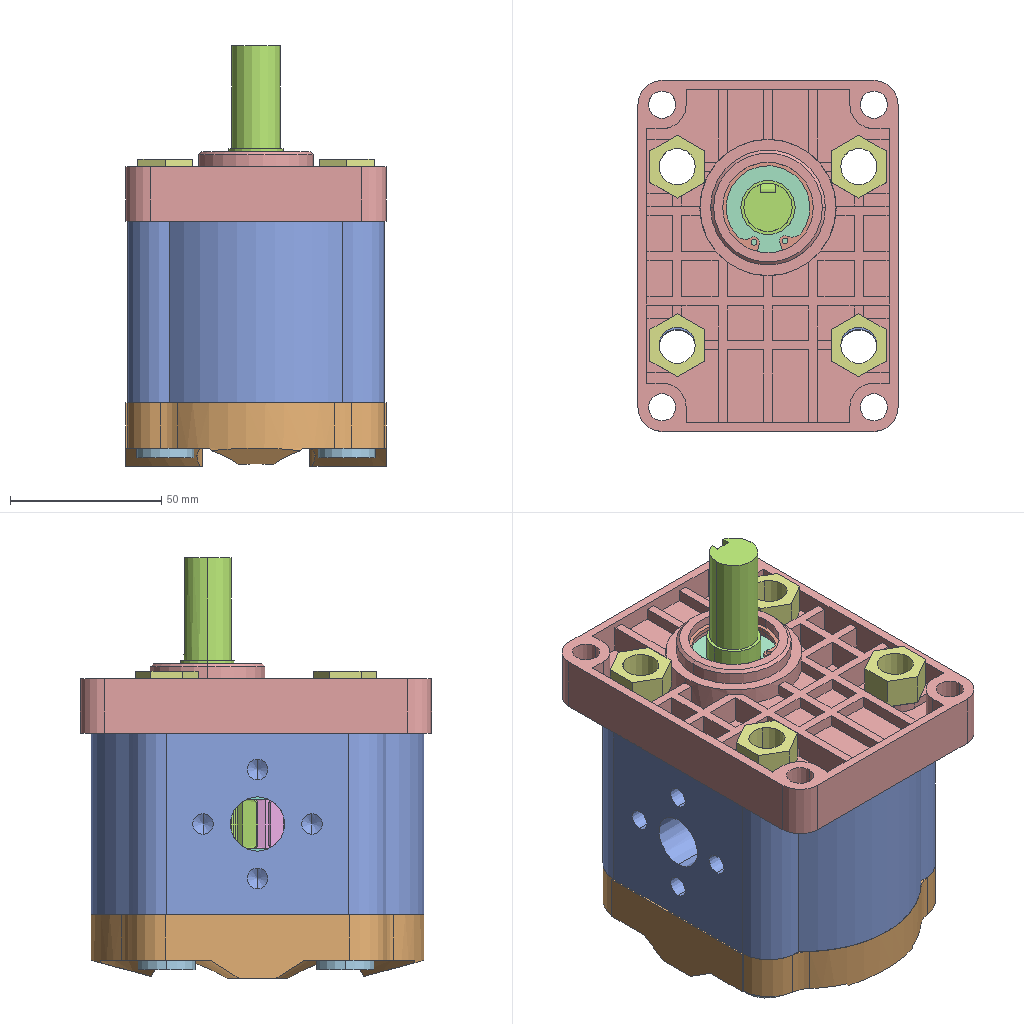Assembly | SolidWorks | 14 different items | 25 placed | box 86 x 116 x 139 mm
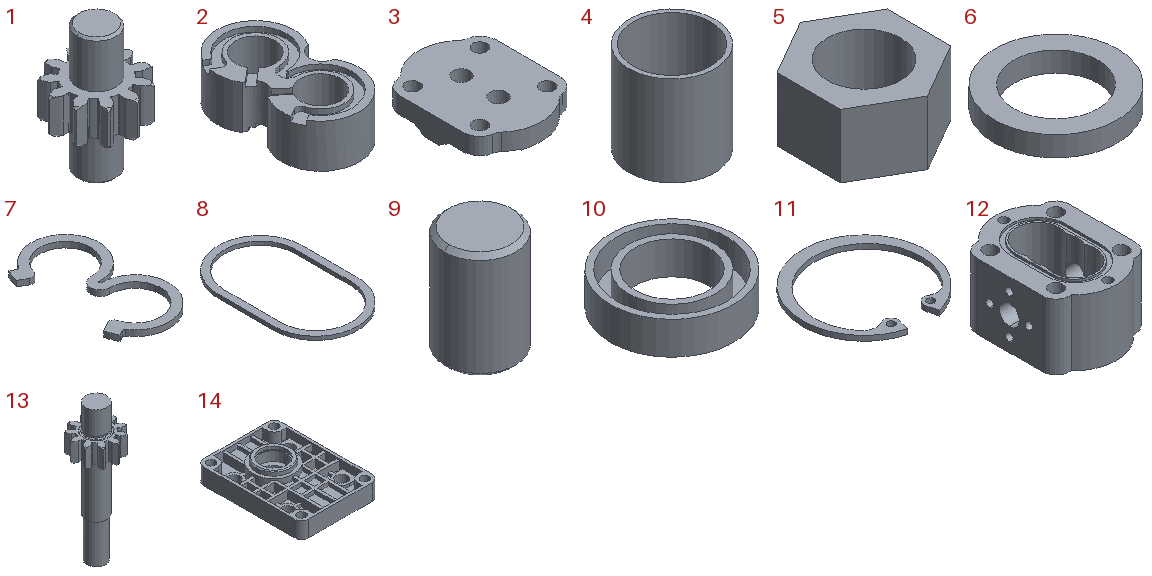Parts list (item | quantity | size | volume | features):
1 | x1 | 38.703 x 38.313 x 59 mm | 23395 mm3 | features ICE 3, Chamfer 2, CirPattern 2, Fillet 2, Extrusion 1
2 | x2 | 39 x 72 x 22 mm | 33796 mm3 | features ICE 4, Extrusion 1, Fillet 1, MirrorPattern 1
3 | x1 | 86 x 110 x 21 mm | 130372 mm3 | features ICE 7, Split 3, HoleWzd 2, MirrorPattern 2, BlendCut 1, Extrusion 1, Fillet 1, MirrorSolid 1, MoveFace 1
4 | x2 | 20 x 20 x 21 mm | 1253 mm3 | features Extrusion 1
5 | x4 | 18 x 20.785 x 10.4 mm | 1742 mm3 | features Extrusion 1
6 | x4 | 19 x 19 x 3.1 mm | 467.469 mm3 | features Extrusion 1
7 | x2 | 35.068 x 65 x 2.7 mm | 1587 mm3 | features Extrusion 1
8 | x2 | 50 x 83 x 2.2 mm | 1853 mm3 | features Extrusion 1
9 | x2 | 8 x 8 x 12 mm | 597.164 mm3 | features Chamfer 1, Extrusion 1
10 | x1 | 30 x 30 x 8 mm | 2262 mm3 | features Extrusion 1, ICE 1
11 | x1 | 31.9 x 31.357 x 1.3 mm | 270.021 mm3 | features Extrusion 1
12 | x1 | 85 x 110 x 60 mm | 286652 mm3 | features ICE 7, HoleWzd 3, MirrorPattern 3, Split 2, BlendCut 1, Extrusion 1, Fillet 1, MoveFace 1
13 | x1 | 38.703 x 38.313 x 117.5 mm | 35920 mm3 | features ICE 5, Fillet 3, CirPattern 2, Chamfer 1, Extrusion 1, RevCut 1
14 | x1 | 86 x 116 x 23 mm | 111724 mm3 | features ICE 11, BossThin 2, Chamfer 1, Extrusion 1, HoleWzd 1, MirrorPattern 1, MoveFace 1, Split 1
Mates (type | each side: item.copy, entity, surface, feature):
Concentric | 12.1 face cylinder Cut-Extrude3 | 3.1 face cylinder Mirror3
Concentric | 14.1 face cylinder Cut-Extrude5 | 13.1 face cylinder Boss-Extrude3
Concentric | 2.1 face cylinder Boss-Extrude1 | 7.1 edge
Concentric | 2.1 edge | 7.1 edge
Coincident | 2.1 face plane Cut-Extrude1 | 7.1 face plane Boss-Extrude1
Concentric | 12.1 face cylinder Cut-Extrude6 | 2.1 face cylinder Boss-Extrude1 | 2 times
Concentric | 12.1 face cylinder Mirror3 | 8.1 face cylinder Boss-Extrude1 | 2 times
Coincident | 12.1 face plane Mirror3 | 8.1 face plane Boss-Extrude1
Concentric | 12.1 face cylinder Cut-Extrude6 | 13.1 face cylinder Boss-Extrude1
Concentric | 12.1 face cylinder Cut-Extrude6 | 1.1 face cylinder Boss-Extrude2
Coincident | 13.1 face plane Blank | 1.1 face plane Blank
Coincident | 12.1 face plane Boss-Extrude1 | 2.1 face plane Boss-Extrude1
Concentric | 14.1 face cylinder Cut-Extrude8 | 11.1 edge
Coincident | 14.1 face plane Cut-Extrude8 | 11.1 face plane Boss-Extrude1
Parallel | 14.1 face plane Boss-Extrude1 | 12.1 face plane Boss-Extrude1
Parallel | 12.1 face plane Boss-Extrude1 | 3.1 face plane Mirror3
Coincident | 14.1 edge | 9.1 face plane Boss-Extrude1
Concentric | 14.1 face cylinder Ø8.0mm blind dowel hole 1 | 9.1 face cylinder Boss-Extrude1
Coincident | 14.1 edge | 9.2 face plane Boss-Extrude1
Concentric | 14.1 face cylinder Ø8.0mm blind dowel hole 1 | 9.2 face cylinder Boss-Extrude1
Coincident | 12.1 plane | 13.1 plane
GearDim | 13.1 select_type:24 | 1.1 select_type:24
Concentric | 13.1 face cylinder Boss-Extrude1 | 4.1 face cylinder Boss-Extrude1
Coincident | 13.1 face plane Cut-Revolve1 | 4.1 face plane Boss-Extrude1
Concentric | 1.1 face cylinder Boss-Extrude2 | 4.2 face cylinder Boss-Extrude1
Coincident | 1.1 face plane Blank | 4.2 face plane Boss-Extrude1
Coincident | 14.1 face plane Boss-Extrude1 | 12.1 face plane Boss-Extrude1
Coincident | 14.1 face plane Cut-Extrude7 | 10.1 face plane Boss-Extrude1
Concentric | 13.1 face cylinder Boss-Extrude3 | 10.1 face cylinder Boss-Extrude1
Coincident | 12.1 face plane Boss-Extrude1 | 3.1 face plane Boss-Extrude1
Concentric | 3.1 face cylinder Hole1 | 6.1 face cylinder Boss-Extrude1
Coincident | 3.1 face plane Cut-Loft1 | 6.1 face plane Boss-Extrude1
Concentric | 3.1 face cylinder Hole1 | assembly face
Coincident | 6.1 face plane Boss-Extrude1 | assembly face
Concentric | 5.1 face cylinder Boss-Extrude1 | assembly face
Coincident | 14.1 face plane Mirror1 | 5.1 face plane Boss-Extrude1
Parallel | 14.1 face plane Boss-Extrude1 | 5.1 face plane Boss-Extrude1
Parallel | 13.1 plane | assembly plane
Coincident | 13.1 plane | assembly plane